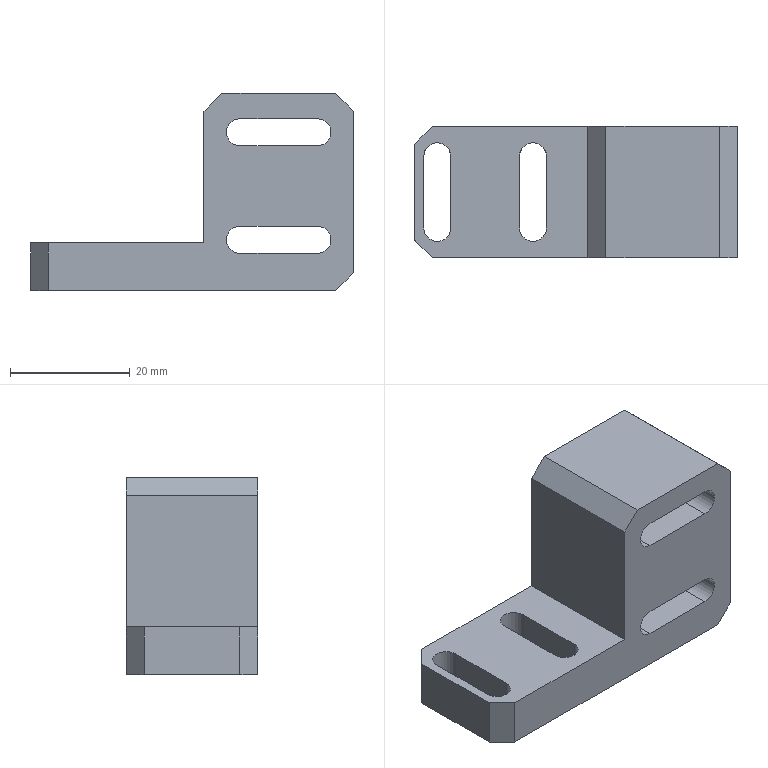Part | STEP file | 0-19 Finger cylinder fixed plate 12 | 1 solid | 29 faces | box 54 x 22 x 33 mm | volume 18493 mm3 | plane 21 | cylinder 8 | commonest cylinder face diameters 4.5 x8